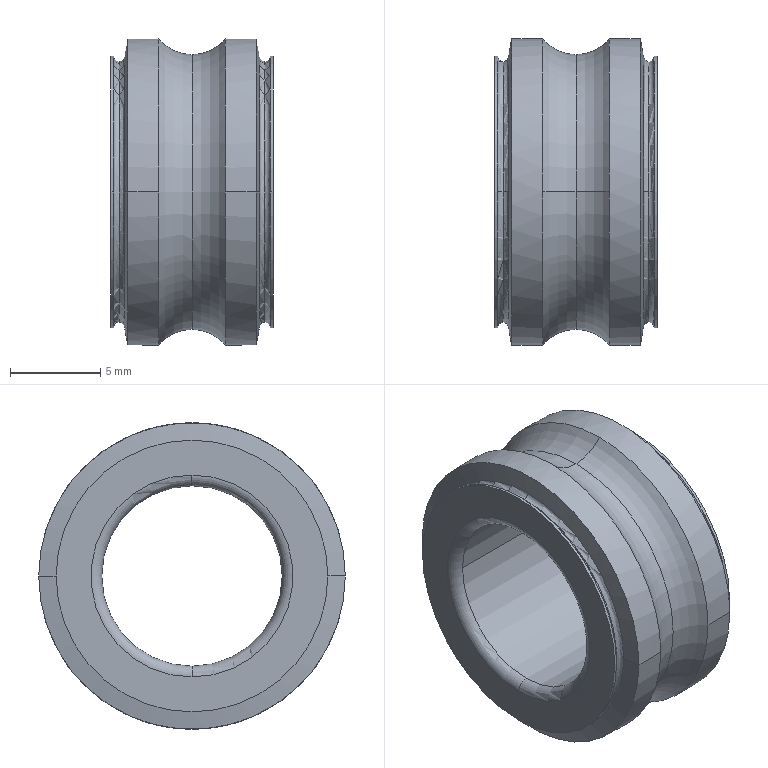Part | SolidWorks | features BaseBody 1 | 1 solid | 32 faces | box 9 x 17 x 17 mm | volume 1119 mm3 | torus 16 | cylinder 10 | cone 4 | plane 2 | commonest cylinder face diameters 15.07 x4 17 x4 10 x2
STEP:
#1=CARTESIAN_POINT('',(6.349,8.5,0.));
#2=VERTEX_POINT('',#1);
#3=CARTESIAN_POINT('',(8.065,8.5,0.));
#4=VERTEX_POINT('',#3);
#5=CARTESIAN_POINT('',(7.207,8.5,0.));
#6=DIRECTION('',(1.,0.,0.));
#7=VECTOR('',#6,1000.);
#8=LINE('',#5,#7);
#9=EDGE_CURVE('',#2,#4,#8,.T.);
#10=ORIENTED_EDGE('',*,*,#9,.T.);
#11=CARTESIAN_POINT('',(8.065,-8.5,0.));
#12=VERTEX_POINT('',#11);
#13=CARTESIAN_POINT('',(8.065,0.,0.));
#14=DIRECTION('',(1.,0.,0.));
#15=DIRECTION('',(0.,1.,0.));
#16=AXIS2_PLACEMENT_3D('',#13,#14,#15);
#17=CIRCLE('',#16,8.5);
#18=EDGE_CURVE('',#12,#4,#17,.T.);
#19=ORIENTED_EDGE('',*,*,#18,.F.);
#20=CARTESIAN_POINT('',(6.349,-8.5,0.));
#21=VERTEX_POINT('',#20);
#22=CARTESIAN_POINT('',(7.207,-8.5,0.));
#23=DIRECTION('',(-1.,0.,0.));
#24=VECTOR('',#23,1000.);
#25=LINE('',#22,#24);
#26=EDGE_CURVE('',#12,#21,#25,.T.);
#27=ORIENTED_EDGE('',*,*,#26,.T.);
#28=CARTESIAN_POINT('',(6.349,0.,-8.5));
#29=VERTEX_POINT('',#28);
#30=CARTESIAN_POINT('',(6.349,0.,0.));
#31=DIRECTION('',(1.,0.,0.));
#32=DIRECTION('',(0.,1.,0.));
#33=AXIS2_PLACEMENT_3D('',#30,#31,#32);
#34=CIRCLE('',#33,8.5);
#35=EDGE_CURVE('',#21,#29,#34,.T.);
#36=ORIENTED_EDGE('',*,*,#35,.T.);
#37=CARTESIAN_POINT('',(6.349,0.,0.));
#38=DIRECTION('',(1.,0.,0.));
#39=DIRECTION('',(0.,1.,0.));
#40=AXIS2_PLACEMENT_3D('',#37,#38,#39);
#41=CIRCLE('',#40,8.5);
#42=EDGE_CURVE('',#29,#2,#41,.T.);
#43=ORIENTED_EDGE('',*,*,#42,.T.);
#44=EDGE_LOOP('',(#10,#19,#27,#36,#43));
#45=FACE_OUTER_BOUND('',#44,.T.);
#46=CARTESIAN_POINT('',(7.207,0.,0.));
#47=DIRECTION('',(1.,0.,0.));
#48=DIRECTION('',(0.,1.,0.));
#49=AXIS2_PLACEMENT_3D('',#46,#47,#48);
#50=CYLINDRICAL_SURFACE('',#49,8.5);
#51=ADVANCED_FACE('',(#45),#50,.T.);
#52=CARTESIAN_POINT('',(4.5,0.,7.619));
#53=VERTEX_POINT('',#52);
#54=CARTESIAN_POINT('',(4.5,0.,-7.619));
#55=VERTEX_POINT('',#54);
#56=CARTESIAN_POINT('',(4.5,0.,0.));
#57=DIRECTION('',(-1.,0.,0.));
#58=DIRECTION('',(0.,0.,1.));
#59=AXIS2_PLACEMENT_3D('',#56,#57,#58);
#60=CIRCLE('',#59,7.619);
#61=EDGE_CURVE('',#53,#55,#60,.T.);
#62=ORIENTED_EDGE('',*,*,#61,.T.);
#63=CARTESIAN_POINT('',(2.651,0.,-8.5));
#64=VERTEX_POINT('',#63);
#65=CARTESIAN_POINT('',(4.5,0.,-10.));
#66=DIRECTION('',(0.,-1.,0.));
#67=DIRECTION('',(0.,0.,-1.));
#68=AXIS2_PLACEMENT_3D('',#65,#66,#67);
#69=CIRCLE('',#68,2.381);
#70=EDGE_CURVE('',#55,#64,#69,.T.);
#71=ORIENTED_EDGE('',*,*,#70,.T.);
#72=CARTESIAN_POINT('',(2.651,8.5,0.));
#73=VERTEX_POINT('',#72);
#74=CARTESIAN_POINT('',(2.651,0.,0.));
#75=DIRECTION('',(1.,0.,0.));
#76=DIRECTION('',(0.,1.,0.));
#77=AXIS2_PLACEMENT_3D('',#74,#75,#76);
#78=CIRCLE('',#77,8.5);
#79=EDGE_CURVE('',#64,#73,#78,.T.);
#80=ORIENTED_EDGE('',*,*,#79,.T.);
#81=CARTESIAN_POINT('',(2.651,0.,8.5));
#82=VERTEX_POINT('',#81);
#83=CARTESIAN_POINT('',(2.651,0.,0.));
#84=DIRECTION('',(1.,0.,0.));
#85=DIRECTION('',(0.,1.,0.));
#86=AXIS2_PLACEMENT_3D('',#83,#84,#85);
#87=CIRCLE('',#86,8.5);
#88=EDGE_CURVE('',#73,#82,#87,.T.);
#89=ORIENTED_EDGE('',*,*,#88,.T.);
#90=CARTESIAN_POINT('',(4.5,0.,10.));
#91=DIRECTION('',(0.,-1.,0.));
#92=DIRECTION('',(0.,0.,1.));
#93=AXIS2_PLACEMENT_3D('',#90,#91,#92);
#94=CIRCLE('',#93,2.381);
#95=EDGE_CURVE('',#82,#53,#94,.T.);
#96=ORIENTED_EDGE('',*,*,#95,.T.);
#97=EDGE_LOOP('',(#62,#71,#80,#89,#96));
#98=FACE_OUTER_BOUND('',#97,.T.);
#99=CARTESIAN_POINT('',(4.5,0.,0.));
#100=DIRECTION('',(1.,0.,0.));
#101=DIRECTION('',(0.,0.,-1.));
#102=AXIS2_PLACEMENT_3D('',#99,#100,#101);
#103=TOROIDAL_SURFACE('',#102,10.,2.381);
#104=ADVANCED_FACE('',(#98),#103,.F.);
#105=CARTESIAN_POINT('',(0.9348,8.5,0.));
#106=VERTEX_POINT('',#105);
#107=CARTESIAN_POINT('',(1.793,8.5,0.));
#108=DIRECTION('',(1.,0.,0.));
#109=VECTOR('',#108,1000.);
#110=LINE('',#107,#109);
#111=EDGE_CURVE('',#106,#73,#110,.T.);
#112=ORIENTED_EDGE('',*,*,#111,.T.);
#113=ORIENTED_EDGE('',*,*,#79,.F.);
#114=CARTESIAN_POINT('',(2.651,-8.5,0.));
#115=VERTEX_POINT('',#114);
#116=CARTESIAN_POINT('',(2.651,0.,0.));
#117=DIRECTION('',(1.,0.,0.));
#118=DIRECTION('',(0.,1.,0.));
#119=AXIS2_PLACEMENT_3D('',#116,#117,#118);
#120=CIRCLE('',#119,8.5);
#121=EDGE_CURVE('',#115,#64,#120,.T.);
#122=ORIENTED_EDGE('',*,*,#121,.F.);
#123=CARTESIAN_POINT('',(0.9348,-8.5,0.));
#124=VERTEX_POINT('',#123);
#125=CARTESIAN_POINT('',(1.793,-8.5,0.));
#126=DIRECTION('',(-1.,0.,0.));
#127=VECTOR('',#126,1000.);
#128=LINE('',#125,#127);
#129=EDGE_CURVE('',#115,#124,#128,.T.);
#130=ORIENTED_EDGE('',*,*,#129,.T.);
#131=CARTESIAN_POINT('',(0.9348,0.,0.));
#132=DIRECTION('',(1.,0.,0.));
#133=DIRECTION('',(0.,1.,0.));
#134=AXIS2_PLACEMENT_3D('',#131,#132,#133);
#135=CIRCLE('',#134,8.5);
#136=EDGE_CURVE('',#124,#106,#135,.T.);
#137=ORIENTED_EDGE('',*,*,#136,.T.);
#138=EDGE_LOOP('',(#112,#113,#122,#130,#137));
#139=FACE_OUTER_BOUND('',#138,.T.);
#140=CARTESIAN_POINT('',(1.793,0.,0.));
#141=DIRECTION('',(1.,0.,0.));
#142=DIRECTION('',(0.,1.,0.));
#143=AXIS2_PLACEMENT_3D('',#140,#141,#142);
#144=CYLINDRICAL_SURFACE('',#143,8.5);
#145=ADVANCED_FACE('',(#139),#144,.T.);
#146=CARTESIAN_POINT('',(0.7554,7.482,0.));
#147=VERTEX_POINT('',#146);
#148=CARTESIAN_POINT('',(0.8451,7.991,0.));
#149=DIRECTION('',(0.1736,0.9848,0.));
#150=VECTOR('',#149,1000.);
#151=LINE('',#148,#150);
#152=EDGE_CURVE('',#147,#106,#151,.T.);
#153=ORIENTED_EDGE('',*,*,#152,.T.);
#154=ORIENTED_EDGE('',*,*,#136,.F.);
#155=CARTESIAN_POINT('',(0.7554,-7.482,0.));
#156=VERTEX_POINT('',#155);
#157=CARTESIAN_POINT('',(0.8451,-7.991,0.));
#158=DIRECTION('',(-0.1736,0.9848,0.));
#159=VECTOR('',#158,1000.);
#160=LINE('',#157,#159);
#161=EDGE_CURVE('',#124,#156,#160,.T.);
#162=ORIENTED_EDGE('',*,*,#161,.T.);
#163=CARTESIAN_POINT('',(0.7554,0.,-7.482));
#164=VERTEX_POINT('',#163);
#165=CARTESIAN_POINT('',(0.7554,0.,0.));
#166=DIRECTION('',(1.,0.,0.));
#167=DIRECTION('',(0.,1.,0.));
#168=AXIS2_PLACEMENT_3D('',#165,#166,#167);
#169=CIRCLE('',#168,7.482);
#170=EDGE_CURVE('',#156,#164,#169,.T.);
#171=ORIENTED_EDGE('',*,*,#170,.T.);
#172=CARTESIAN_POINT('',(0.7554,0.,0.));
#173=DIRECTION('',(1.,0.,0.));
#174=DIRECTION('',(0.,1.,0.));
#175=AXIS2_PLACEMENT_3D('',#172,#173,#174);
#176=CIRCLE('',#175,7.482);
#177=EDGE_CURVE('',#164,#147,#176,.T.);
#178=ORIENTED_EDGE('',*,*,#177,.T.);
#179=EDGE_LOOP('',(#153,#154,#162,#171,#178));
#180=FACE_OUTER_BOUND('',#179,.T.);
#181=CARTESIAN_POINT('',(0.8451,0.,0.));
#182=DIRECTION('',(1.,0.,0.));
#183=DIRECTION('',(0.,1.,0.));
#184=AXIS2_PLACEMENT_3D('',#181,#182,#183);
#185=CONICAL_SURFACE('',#184,7.991,1.396);
#186=ADVANCED_FACE('',(#180),#185,.T.);
#187=CARTESIAN_POINT('',(0.456,0.,7.231));
#188=VERTEX_POINT('',#187);
#189=CARTESIAN_POINT('',(0.456,0.,-7.231));
#190=VERTEX_POINT('',#189);
#191=CARTESIAN_POINT('',(0.456,0.,0.));
#192=DIRECTION('',(-1.,0.,0.));
#193=DIRECTION('',(0.,0.,1.));
#194=AXIS2_PLACEMENT_3D('',#191,#192,#193);
#195=CIRCLE('',#194,7.231);
#196=EDGE_CURVE('',#188,#190,#195,.T.);
#197=ORIENTED_EDGE('',*,*,#196,.T.);
#198=CARTESIAN_POINT('',(0.152,0.,-7.535));
#199=VERTEX_POINT('',#198);
#200=CARTESIAN_POINT('',(0.456,0.,-7.535));
#201=DIRECTION('',(0.,-1.,0.));
#202=DIRECTION('',(0.,0.,-1.));
#203=AXIS2_PLACEMENT_3D('',#200,#201,#202);
#204=CIRCLE('',#203,0.304);
#205=EDGE_CURVE('',#190,#199,#204,.T.);
#206=ORIENTED_EDGE('',*,*,#205,.T.);
#207=CARTESIAN_POINT('',(0.152,7.535,0.));
#208=VERTEX_POINT('',#207);
#209=CARTESIAN_POINT('',(0.152,0.,0.));
#210=DIRECTION('',(1.,0.,0.));
#211=DIRECTION('',(0.,1.,0.));
#212=AXIS2_PLACEMENT_3D('',#209,#210,#211);
#213=CIRCLE('',#212,7.535);
#214=EDGE_CURVE('',#199,#208,#213,.T.);
#215=ORIENTED_EDGE('',*,*,#214,.T.);
#216=CARTESIAN_POINT('',(0.152,0.,7.535));
#217=VERTEX_POINT('',#216);
#218=CARTESIAN_POINT('',(0.152,0.,0.));
#219=DIRECTION('',(1.,0.,0.));
#220=DIRECTION('',(0.,1.,0.));
#221=AXIS2_PLACEMENT_3D('',#218,#219,#220);
#222=CIRCLE('',#221,7.535);
#223=EDGE_CURVE('',#208,#217,#222,.T.);
#224=ORIENTED_EDGE('',*,*,#223,.T.);
#225=CARTESIAN_POINT('',(0.456,0.,7.535));
#226=DIRECTION('',(0.,-1.,0.));
#227=DIRECTION('',(0.,0.,1.));
#228=AXIS2_PLACEMENT_3D('',#225,#226,#227);
#229=CIRCLE('',#228,0.304);
#230=EDGE_CURVE('',#217,#188,#229,.T.);
#231=ORIENTED_EDGE('',*,*,#230,.T.);
#232=EDGE_LOOP('',(#197,#206,#215,#224,#231));
#233=FACE_OUTER_BOUND('',#232,.T.);
#234=CARTESIAN_POINT('',(0.456,0.,0.));
#235=DIRECTION('',(1.,0.,0.));
#236=DIRECTION('',(0.,0.,-1.));
#237=AXIS2_PLACEMENT_3D('',#234,#235,#236);
#238=TOROIDAL_SURFACE('',#237,7.535,0.304);
#239=ADVANCED_FACE('',(#233),#238,.F.);
#240=CARTESIAN_POINT('',(0.,7.535,0.));
#241=VERTEX_POINT('',#240);
#242=CARTESIAN_POINT('',(0.076,7.535,0.));
#243=DIRECTION('',(1.,0.,0.));
#244=VECTOR('',#243,1000.);
#245=LINE('',#242,#244);
#246=EDGE_CURVE('',#241,#208,#245,.T.);
#247=ORIENTED_EDGE('',*,*,#246,.T.);
#248=ORIENTED_EDGE('',*,*,#214,.F.);
#249=CARTESIAN_POINT('',(0.152,-7.535,0.));
#250=VERTEX_POINT('',#249);
#251=CARTESIAN_POINT('',(0.152,0.,0.));
#252=DIRECTION('',(1.,0.,0.));
#253=DIRECTION('',(0.,1.,0.));
#254=AXIS2_PLACEMENT_3D('',#251,#252,#253);
#255=CIRCLE('',#254,7.535);
#256=EDGE_CURVE('',#250,#199,#255,.T.);
#257=ORIENTED_EDGE('',*,*,#256,.F.);
#258=CARTESIAN_POINT('',(0.,-7.535,0.));
#259=VERTEX_POINT('',#258);
#260=CARTESIAN_POINT('',(0.076,-7.535,0.));
#261=DIRECTION('',(-1.,0.,0.));
#262=VECTOR('',#261,1000.);
#263=LINE('',#260,#262);
#264=EDGE_CURVE('',#250,#259,#263,.T.);
#265=ORIENTED_EDGE('',*,*,#264,.T.);
#266=CARTESIAN_POINT('',(0.,0.,0.));
#267=DIRECTION('',(1.,0.,0.));
#268=DIRECTION('',(0.,1.,0.));
#269=AXIS2_PLACEMENT_3D('',#266,#267,#268);
#270=CIRCLE('',#269,7.535);
#271=EDGE_CURVE('',#259,#241,#270,.T.);
#272=ORIENTED_EDGE('',*,*,#271,.T.);
#273=EDGE_LOOP('',(#247,#248,#257,#265,#272));
#274=FACE_OUTER_BOUND('',#273,.T.);
#275=CARTESIAN_POINT('',(0.076,0.,0.));
#276=DIRECTION('',(1.,0.,0.));
#277=DIRECTION('',(0.,1.,0.));
#278=AXIS2_PLACEMENT_3D('',#275,#276,#277);
#279=CYLINDRICAL_SURFACE('',#278,7.535);
#280=ADVANCED_FACE('',(#274),#279,.T.);
#281=CARTESIAN_POINT('',(0.,0.,5.6));
#282=VERTEX_POINT('',#281);
#283=CARTESIAN_POINT('',(0.,0.,-5.6));
#284=VERTEX_POINT('',#283);
#285=CARTESIAN_POINT('',(0.,0.,0.));
#286=DIRECTION('',(1.,0.,0.));
#287=DIRECTION('',(0.,1.,0.));
#288=AXIS2_PLACEMENT_3D('',#285,#286,#287);
#289=CIRCLE('',#288,5.6);
#290=EDGE_CURVE('',#282,#284,#289,.T.);
#291=ORIENTED_EDGE('',*,*,#290,.T.);
#292=CARTESIAN_POINT('',(0.,0.,0.));
#293=DIRECTION('',(1.,0.,0.));
#294=DIRECTION('',(0.,1.,0.));
#295=AXIS2_PLACEMENT_3D('',#292,#293,#294);
#296=CIRCLE('',#295,5.6);
#297=EDGE_CURVE('',#284,#282,#296,.T.);
#298=ORIENTED_EDGE('',*,*,#297,.T.);
#299=EDGE_LOOP('',(#291,#298));
#300=FACE_BOUND('',#299,.T.);
#301=CARTESIAN_POINT('',(0.,0.,0.));
#302=DIRECTION('',(1.,0.,0.));
#303=DIRECTION('',(0.,1.,0.));
#304=AXIS2_PLACEMENT_3D('',#301,#302,#303);
#305=CIRCLE('',#304,7.535);
#306=EDGE_CURVE('',#241,#259,#305,.T.);
#307=ORIENTED_EDGE('',*,*,#306,.F.);
#308=ORIENTED_EDGE('',*,*,#271,.F.);
#309=EDGE_LOOP('',(#307,#308));
#310=FACE_OUTER_BOUND('',#309,.T.);
#311=CARTESIAN_POINT('',(0.,6.568,0.));
#312=DIRECTION('',(-1.,0.,0.));
#313=DIRECTION('',(0.,0.,1.));
#314=AXIS2_PLACEMENT_3D('',#311,#312,#313);
#315=PLANE('',#314);
#316=ADVANCED_FACE('',(#300,#310),#315,.T.);
#317=CARTESIAN_POINT('',(0.6,0.,-5.));
#318=VERTEX_POINT('',#317);
#319=CARTESIAN_POINT('',(0.6,0.,-5.6));
#320=DIRECTION('',(0.,-1.,0.));
#321=DIRECTION('',(0.,0.,-1.));
#322=AXIS2_PLACEMENT_3D('',#319,#320,#321);
#323=CIRCLE('',#322,0.6);
#324=EDGE_CURVE('',#318,#284,#323,.T.);
#325=ORIENTED_EDGE('',*,*,#324,.T.);
#326=ORIENTED_EDGE('',*,*,#290,.F.);
#327=CARTESIAN_POINT('',(0.6,0.,5.));
#328=VERTEX_POINT('',#327);
#329=CARTESIAN_POINT('',(0.6,0.,5.6));
#330=DIRECTION('',(0.,-1.,0.));
#331=DIRECTION('',(0.,0.,1.));
#332=AXIS2_PLACEMENT_3D('',#329,#330,#331);
#333=CIRCLE('',#332,0.6);
#334=EDGE_CURVE('',#282,#328,#333,.T.);
#335=ORIENTED_EDGE('',*,*,#334,.T.);
#336=CARTESIAN_POINT('',(0.6,-5.,0.));
#337=VERTEX_POINT('',#336);
#338=CARTESIAN_POINT('',(0.6,0.,0.));
#339=DIRECTION('',(1.,0.,0.));
#340=DIRECTION('',(0.,1.,0.));
#341=AXIS2_PLACEMENT_3D('',#338,#339,#340);
#342=CIRCLE('',#341,5.);
#343=EDGE_CURVE('',#328,#337,#342,.T.);
#344=ORIENTED_EDGE('',*,*,#343,.T.);
#345=CARTESIAN_POINT('',(0.6,0.,0.));
#346=DIRECTION('',(1.,0.,0.));
#347=DIRECTION('',(0.,1.,0.));
#348=AXIS2_PLACEMENT_3D('',#345,#346,#347);
#349=CIRCLE('',#348,5.);
#350=EDGE_CURVE('',#337,#318,#349,.T.);
#351=ORIENTED_EDGE('',*,*,#350,.T.);
#352=EDGE_LOOP('',(#325,#326,#335,#344,#351));
#353=FACE_OUTER_BOUND('',#352,.T.);
#354=CARTESIAN_POINT('',(0.6,0.,0.));
#355=DIRECTION('',(1.,0.,0.));
#356=DIRECTION('',(0.,0.,-1.));
#357=AXIS2_PLACEMENT_3D('',#354,#355,#356);
#358=TOROIDAL_SURFACE('',#357,5.6,0.6);
#359=ADVANCED_FACE('',(#353),#358,.T.);
#360=CARTESIAN_POINT('',(0.6,5.,0.));
#361=VERTEX_POINT('',#360);
#362=CARTESIAN_POINT('',(8.4,5.,0.));
#363=VERTEX_POINT('',#362);
#364=CARTESIAN_POINT('',(4.5,5.,0.));
#365=DIRECTION('',(1.,0.,0.));
#366=VECTOR('',#365,1000.);
#367=LINE('',#364,#366);
#368=EDGE_CURVE('',#361,#363,#367,.T.);
#369=ORIENTED_EDGE('',*,*,#368,.T.);
#370=CARTESIAN_POINT('',(8.4,0.,5.));
#371=VERTEX_POINT('',#370);
#372=CARTESIAN_POINT('',(8.4,0.,0.));
#373=DIRECTION('',(1.,0.,0.));
#374=DIRECTION('',(0.,1.,0.));
#375=AXIS2_PLACEMENT_3D('',#372,#373,#374);
#376=CIRCLE('',#375,5.);
#377=EDGE_CURVE('',#363,#371,#376,.T.);
#378=ORIENTED_EDGE('',*,*,#377,.T.);
#379=CARTESIAN_POINT('',(8.4,-5.,0.));
#380=VERTEX_POINT('',#379);
#381=CARTESIAN_POINT('',(8.4,0.,0.));
#382=DIRECTION('',(1.,0.,0.));
#383=DIRECTION('',(0.,1.,0.));
#384=AXIS2_PLACEMENT_3D('',#381,#382,#383);
#385=CIRCLE('',#384,5.);
#386=EDGE_CURVE('',#371,#380,#385,.T.);
#387=ORIENTED_EDGE('',*,*,#386,.T.);
#388=CARTESIAN_POINT('',(4.5,-5.,0.));
#389=DIRECTION('',(-1.,0.,0.));
#390=VECTOR('',#389,1000.);
#391=LINE('',#388,#390);
#392=EDGE_CURVE('',#380,#337,#391,.T.);
#393=ORIENTED_EDGE('',*,*,#392,.T.);
#394=ORIENTED_EDGE('',*,*,#343,.F.);
#395=CARTESIAN_POINT('',(0.6,0.,0.));
#396=DIRECTION('',(1.,0.,0.));
#397=DIRECTION('',(0.,1.,0.));
#398=AXIS2_PLACEMENT_3D('',#395,#396,#397);
#399=CIRCLE('',#398,5.);
#400=EDGE_CURVE('',#361,#328,#399,.T.);
#401=ORIENTED_EDGE('',*,*,#400,.F.);
#402=EDGE_LOOP('',(#369,#378,#387,#393,#394,#401));
#403=FACE_OUTER_BOUND('',#402,.T.);
#404=CARTESIAN_POINT('',(4.5,0.,0.));
#405=DIRECTION('',(1.,0.,0.));
#406=DIRECTION('',(0.,1.,0.));
#407=AXIS2_PLACEMENT_3D('',#404,#405,#406);
#408=CYLINDRICAL_SURFACE('',#407,5.);
#409=ADVANCED_FACE('',(#403),#408,.F.);
#410=CARTESIAN_POINT('',(9.,0.,-5.6));
#411=VERTEX_POINT('',#410);
#412=CARTESIAN_POINT('',(8.4,0.,-5.));
#413=VERTEX_POINT('',#412);
#414=CARTESIAN_POINT('',(8.4,0.,-5.6));
#415=DIRECTION('',(0.,-1.,0.));
#416=DIRECTION('',(0.,0.,-1.));
#417=AXIS2_PLACEMENT_3D('',#414,#415,#416);
#418=CIRCLE('',#417,0.6);
#419=EDGE_CURVE('',#411,#413,#418,.T.);
#420=ORIENTED_EDGE('',*,*,#419,.T.);
#421=CARTESIAN_POINT('',(8.4,0.,0.));
#422=DIRECTION('',(1.,0.,0.));
#423=DIRECTION('',(0.,1.,0.));
#424=AXIS2_PLACEMENT_3D('',#421,#422,#423);
#425=CIRCLE('',#424,5.);
#426=EDGE_CURVE('',#380,#413,#425,.T.);
#427=ORIENTED_EDGE('',*,*,#426,.F.);
#428=ORIENTED_EDGE('',*,*,#386,.F.);
#429=CARTESIAN_POINT('',(9.,0.,5.6));
#430=VERTEX_POINT('',#429);
#431=CARTESIAN_POINT('',(8.4,0.,5.6));
#432=DIRECTION('',(0.,-1.,0.));
#433=DIRECTION('',(0.,0.,1.));
#434=AXIS2_PLACEMENT_3D('',#431,#432,#433);
#435=CIRCLE('',#434,0.6);
#436=EDGE_CURVE('',#371,#430,#435,.T.);
#437=ORIENTED_EDGE('',*,*,#436,.T.);
#438=CARTESIAN_POINT('',(9.,0.,0.));
#439=DIRECTION('',(1.,0.,0.));
#440=DIRECTION('',(0.,1.,0.));
#441=AXIS2_PLACEMENT_3D('',#438,#439,#440);
#442=CIRCLE('',#441,5.6);
#443=EDGE_CURVE('',#430,#411,#442,.T.);
#444=ORIENTED_EDGE('',*,*,#443,.T.);
#445=EDGE_LOOP('',(#420,#427,#428,#437,#444));
#446=FACE_OUTER_BOUND('',#445,.T.);
#447=CARTESIAN_POINT('',(8.4,0.,0.));
#448=DIRECTION('',(1.,0.,0.));
#449=DIRECTION('',(0.,0.,-1.));
#450=AXIS2_PLACEMENT_3D('',#447,#448,#449);
#451=TOROIDAL_SURFACE('',#450,5.6,0.6);
#452=ADVANCED_FACE('',(#446),#451,.T.);
#453=CARTESIAN_POINT('',(9.,0.,0.));
#454=DIRECTION('',(1.,0.,0.));
#455=DIRECTION('',(0.,1.,0.));
#456=AXIS2_PLACEMENT_3D('',#453,#454,#455);
#457=CIRCLE('',#456,5.6);
#458=EDGE_CURVE('',#411,#430,#457,.T.);
#459=ORIENTED_EDGE('',*,*,#458,.F.);
#460=ORIENTED_EDGE('',*,*,#443,.F.);
#461=EDGE_LOOP('',(#459,#460));
#462=FACE_BOUND('',#461,.T.);
#463=CARTESIAN_POINT('',(9.,7.535,0.));
#464=VERTEX_POINT('',#463);
#465=CARTESIAN_POINT('',(9.,-7.535,0.));
#466=VERTEX_POINT('',#465);
#467=CARTESIAN_POINT('',(9.,0.,0.));
#468=DIRECTION('',(1.,0.,0.));
#469=DIRECTION('',(0.,1.,0.));
#470=AXIS2_PLACEMENT_3D('',#467,#468,#469);
#471=CIRCLE('',#470,7.535);
#472=EDGE_CURVE('',#464,#466,#471,.T.);
#473=ORIENTED_EDGE('',*,*,#472,.T.);
#474=CARTESIAN_POINT('',(9.,0.,0.));
#475=DIRECTION('',(1.,0.,0.));
#476=DIRECTION('',(0.,1.,0.));
#477=AXIS2_PLACEMENT_3D('',#474,#475,#476);
#478=CIRCLE('',#477,7.535);
#479=EDGE_CURVE('',#466,#464,#478,.T.);
#480=ORIENTED_EDGE('',*,*,#479,.T.);
#481=EDGE_LOOP('',(#473,#480));
#482=FACE_OUTER_BOUND('',#481,.T.);
#483=CARTESIAN_POINT('',(9.,6.568,0.));
#484=DIRECTION('',(1.,0.,0.));
#485=DIRECTION('',(0.,1.,0.));
#486=AXIS2_PLACEMENT_3D('',#483,#484,#485);
#487=PLANE('',#486);
#488=ADVANCED_FACE('',(#462,#482),#487,.T.);
#489=CARTESIAN_POINT('',(8.848,7.535,0.));
#490=VERTEX_POINT('',#489);
#491=CARTESIAN_POINT('',(8.924,7.535,0.));
#492=DIRECTION('',(1.,0.,0.));
#493=VECTOR('',#492,1000.);
#494=LINE('',#491,#493);
#495=EDGE_CURVE('',#490,#464,#494,.T.);
#496=ORIENTED_EDGE('',*,*,#495,.T.);
#497=ORIENTED_EDGE('',*,*,#479,.F.);
#498=CARTESIAN_POINT('',(8.848,-7.535,0.));
#499=VERTEX_POINT('',#498);
#500=CARTESIAN_POINT('',(8.924,-7.535,0.));
#501=DIRECTION('',(-1.,0.,0.));
#502=VECTOR('',#501,1000.);
#503=LINE('',#500,#502);
#504=EDGE_CURVE('',#466,#499,#503,.T.);
#505=ORIENTED_EDGE('',*,*,#504,.T.);
#506=CARTESIAN_POINT('',(8.848,0.,-7.535));
#507=VERTEX_POINT('',#506);
#508=CARTESIAN_POINT('',(8.848,0.,0.));
#509=DIRECTION('',(1.,0.,0.));
#510=DIRECTION('',(0.,1.,0.));
#511=AXIS2_PLACEMENT_3D('',#508,#509,#510);
#512=CIRCLE('',#511,7.535);
#513=EDGE_CURVE('',#499,#507,#512,.T.);
#514=ORIENTED_EDGE('',*,*,#513,.T.);
#515=CARTESIAN_POINT('',(8.848,0.,0.));
#516=DIRECTION('',(1.,0.,0.));
#517=DIRECTION('',(0.,1.,0.));
#518=AXIS2_PLACEMENT_3D('',#515,#516,#517);
#519=CIRCLE('',#518,7.535);
#520=EDGE_CURVE('',#507,#490,#519,.T.);
#521=ORIENTED_EDGE('',*,*,#520,.T.);
#522=EDGE_LOOP('',(#496,#497,#505,#514,#521));
#523=FACE_OUTER_BOUND('',#522,.T.);
#524=CARTESIAN_POINT('',(8.924,0.,0.));
#525=DIRECTION('',(1.,0.,0.));
#526=DIRECTION('',(0.,1.,0.));
#527=AXIS2_PLACEMENT_3D('',#524,#525,#526);
#528=CYLINDRICAL_SURFACE('',#527,7.535);
#529=ADVANCED_FACE('',(#523),#528,.T.);
#530=CARTESIAN_POINT('',(8.544,0.,7.231));
#531=VERTEX_POINT('',#530);
#532=CARTESIAN_POINT('',(8.544,0.,-7.231));
#533=VERTEX_POINT('',#532);
#534=CARTESIAN_POINT('',(8.544,0.,0.));
#535=DIRECTION('',(-1.,0.,0.));
#536=DIRECTION('',(0.,0.,1.));
#537=AXIS2_PLACEMENT_3D('',#534,#535,#536);
#538=CIRCLE('',#537,7.231);
#539=EDGE_CURVE('',#531,#533,#538,.T.);
#540=ORIENTED_EDGE('',*,*,#539,.T.);
#541=CARTESIAN_POINT('',(8.245,0.,-7.482));
#542=VERTEX_POINT('',#541);
#543=CARTESIAN_POINT('',(8.544,0.,-7.535));
#544=DIRECTION('',(0.,-1.,0.));
#545=DIRECTION('',(0.,0.,-1.));
#546=AXIS2_PLACEMENT_3D('',#543,#544,#545);
#547=CIRCLE('',#546,0.304);
#548=EDGE_CURVE('',#533,#542,#547,.T.);
#549=ORIENTED_EDGE('',*,*,#548,.T.);
#550=CARTESIAN_POINT('',(8.245,7.482,0.));
#551=VERTEX_POINT('',#550);
#552=CARTESIAN_POINT('',(8.245,0.,0.));
#553=DIRECTION('',(1.,0.,0.));
#554=DIRECTION('',(0.,1.,0.));
#555=AXIS2_PLACEMENT_3D('',#552,#553,#554);
#556=CIRCLE('',#555,7.482);
#557=EDGE_CURVE('',#542,#551,#556,.T.);
#558=ORIENTED_EDGE('',*,*,#557,.T.);
#559=CARTESIAN_POINT('',(8.245,0.,7.482));
#560=VERTEX_POINT('',#559);
#561=CARTESIAN_POINT('',(8.245,0.,0.));
#562=DIRECTION('',(1.,0.,0.));
#563=DIRECTION('',(0.,1.,0.));
#564=AXIS2_PLACEMENT_3D('',#561,#562,#563);
#565=CIRCLE('',#564,7.482);
#566=EDGE_CURVE('',#551,#560,#565,.T.);
#567=ORIENTED_EDGE('',*,*,#566,.T.);
#568=CARTESIAN_POINT('',(8.544,0.,7.535));
#569=DIRECTION('',(0.,-1.,0.));
#570=DIRECTION('',(0.,0.,1.));
#571=AXIS2_PLACEMENT_3D('',#568,#569,#570);
#572=CIRCLE('',#571,0.304);
#573=EDGE_CURVE('',#560,#531,#572,.T.);
#574=ORIENTED_EDGE('',*,*,#573,.T.);
#575=EDGE_LOOP('',(#540,#549,#558,#567,#574));
#576=FACE_OUTER_BOUND('',#575,.T.);
#577=CARTESIAN_POINT('',(8.544,0.,0.));
#578=DIRECTION('',(1.,0.,0.));
#579=DIRECTION('',(0.,0.,-1.));
#580=AXIS2_PLACEMENT_3D('',#577,#578,#579);
#581=TOROIDAL_SURFACE('',#580,7.535,0.304);
#582=ADVANCED_FACE('',(#576),#581,.F.);
#583=CARTESIAN_POINT('',(8.155,7.991,0.));
#584=DIRECTION('',(0.1736,-0.9848,0.));
#585=VECTOR('',#584,1000.);
#586=LINE('',#583,#585);
#587=EDGE_CURVE('',#4,#551,#586,.T.);
#588=ORIENTED_EDGE('',*,*,#587,.T.);
#589=ORIENTED_EDGE('',*,*,#557,.F.);
#590=CARTESIAN_POINT('',(8.245,-7.482,0.));
#591=VERTEX_POINT('',#590);
#592=CARTESIAN_POINT('',(8.245,0.,0.));
#593=DIRECTION('',(1.,0.,0.));
#594=DIRECTION('',(0.,1.,0.));
#595=AXIS2_PLACEMENT_3D('',#592,#593,#594);
#596=CIRCLE('',#595,7.482);
#597=EDGE_CURVE('',#591,#542,#596,.T.);
#598=ORIENTED_EDGE('',*,*,#597,.F.);
#599=CARTESIAN_POINT('',(8.155,-7.991,0.));
#600=DIRECTION('',(-0.1736,-0.9848,0.));
#601=VECTOR('',#600,1000.);
#602=LINE('',#599,#601);
#603=EDGE_CURVE('',#591,#12,#602,.T.);
#604=ORIENTED_EDGE('',*,*,#603,.T.);
#605=ORIENTED_EDGE('',*,*,#18,.T.);
#606=EDGE_LOOP('',(#588,#589,#598,#604,#605));
#607=FACE_OUTER_BOUND('',#606,.T.);
#608=CARTESIAN_POINT('',(8.155,0.,0.));
#609=DIRECTION('',(-1.,0.,0.));
#610=DIRECTION('',(0.,1.,0.));
#611=AXIS2_PLACEMENT_3D('',#608,#609,#610);
#612=CONICAL_SURFACE('',#611,7.991,1.396);
#613=ADVANCED_FACE('',(#607),#612,.T.);
#614=ORIENTED_EDGE('',*,*,#587,.F.);
#615=CARTESIAN_POINT('',(8.065,0.,0.));
#616=DIRECTION('',(1.,0.,0.));
#617=DIRECTION('',(0.,1.,0.));
#618=AXIS2_PLACEMENT_3D('',#615,#616,#617);
#619=CIRCLE('',#618,8.5);
#620=EDGE_CURVE('',#4,#12,#619,.T.);
#621=ORIENTED_EDGE('',*,*,#620,.T.);
#622=ORIENTED_EDGE('',*,*,#603,.F.);
#623=CARTESIAN_POINT('',(8.245,0.,0.));
#624=DIRECTION('',(1.,0.,0.));
#625=DIRECTION('',(0.,1.,0.));
#626=AXIS2_PLACEMENT_3D('',#623,#624,#625);
#627=CIRCLE('',#626,7.482);
#628=EDGE_CURVE('',#560,#591,#627,.T.);
#629=ORIENTED_EDGE('',*,*,#628,.F.);
#630=ORIENTED_EDGE('',*,*,#566,.F.);
#631=EDGE_LOOP('',(#614,#621,#622,#629,#630));
#632=FACE_OUTER_BOUND('',#631,.T.);
#633=CARTESIAN_POINT('',(8.155,0.,0.));
#634=DIRECTION('',(-1.,0.,0.));
#635=DIRECTION('',(0.,1.,0.));
#636=AXIS2_PLACEMENT_3D('',#633,#634,#635);
#637=CONICAL_SURFACE('',#636,7.991,1.396);
#638=ADVANCED_FACE('',(#632),#637,.T.);
#639=CARTESIAN_POINT('',(8.544,0.,0.));
#640=DIRECTION('',(-1.,0.,0.));
#641=DIRECTION('',(0.,0.,1.));
#642=AXIS2_PLACEMENT_3D('',#639,#640,#641);
#643=CIRCLE('',#642,7.231);
#644=EDGE_CURVE('',#533,#531,#643,.T.);
#645=ORIENTED_EDGE('',*,*,#644,.T.);
#646=ORIENTED_EDGE('',*,*,#573,.F.);
#647=ORIENTED_EDGE('',*,*,#628,.T.);
#648=ORIENTED_EDGE('',*,*,#597,.T.);
#649=ORIENTED_EDGE('',*,*,#548,.F.);
#650=EDGE_LOOP('',(#645,#646,#647,#648,#649));
#651=FACE_OUTER_BOUND('',#650,.T.);
#652=CARTESIAN_POINT('',(8.544,0.,0.));
#653=DIRECTION('',(1.,0.,0.));
#654=DIRECTION('',(0.,0.,-1.));
#655=AXIS2_PLACEMENT_3D('',#652,#653,#654);
#656=TOROIDAL_SURFACE('',#655,7.535,0.304);
#657=ADVANCED_FACE('',(#651),#656,.F.);
#658=ORIENTED_EDGE('',*,*,#495,.F.);
#659=CARTESIAN_POINT('',(8.848,0.,7.535));
#660=VERTEX_POINT('',#659);
#661=CARTESIAN_POINT('',(8.848,0.,0.));
#662=DIRECTION('',(1.,0.,0.));
#663=DIRECTION('',(0.,1.,0.));
#664=AXIS2_PLACEMENT_3D('',#661,#662,#663);
#665=CIRCLE('',#664,7.535);
#666=EDGE_CURVE('',#490,#660,#665,.T.);
#667=ORIENTED_EDGE('',*,*,#666,.T.);
#668=CARTESIAN_POINT('',(8.848,0.,0.));
#669=DIRECTION('',(1.,0.,0.));
#670=DIRECTION('',(0.,1.,0.));
#671=AXIS2_PLACEMENT_3D('',#668,#669,#670);
#672=CIRCLE('',#671,7.535);
#673=EDGE_CURVE('',#660,#499,#672,.T.);
#674=ORIENTED_EDGE('',*,*,#673,.T.);
#675=ORIENTED_EDGE('',*,*,#504,.F.);
#676=ORIENTED_EDGE('',*,*,#472,.F.);
#677=EDGE_LOOP('',(#658,#667,#674,#675,#676));
#678=FACE_OUTER_BOUND('',#677,.T.);
#679=CARTESIAN_POINT('',(8.924,0.,0.));
#680=DIRECTION('',(1.,0.,0.));
#681=DIRECTION('',(0.,1.,0.));
#682=AXIS2_PLACEMENT_3D('',#679,#680,#681);
#683=CYLINDRICAL_SURFACE('',#682,7.535);
#684=ADVANCED_FACE('',(#678),#683,.T.);
#685=ORIENTED_EDGE('',*,*,#419,.F.);
#686=ORIENTED_EDGE('',*,*,#458,.T.);
#687=ORIENTED_EDGE('',*,*,#436,.F.);
#688=ORIENTED_EDGE('',*,*,#377,.F.);
#689=CARTESIAN_POINT('',(8.4,0.,0.));
#690=DIRECTION('',(1.,0.,0.));
#691=DIRECTION('',(0.,1.,0.));
#692=AXIS2_PLACEMENT_3D('',#689,#690,#691);
#693=CIRCLE('',#692,5.);
#694=EDGE_CURVE('',#413,#363,#693,.T.);
#695=ORIENTED_EDGE('',*,*,#694,.F.);
#696=EDGE_LOOP('',(#685,#686,#687,#688,#695));
#697=FACE_OUTER_BOUND('',#696,.T.);
#698=CARTESIAN_POINT('',(8.4,0.,0.));
#699=DIRECTION('',(1.,0.,0.));
#700=DIRECTION('',(0.,0.,-1.));
#701=AXIS2_PLACEMENT_3D('',#698,#699,#700);
#702=TOROIDAL_SURFACE('',#701,5.6,0.6);
#703=ADVANCED_FACE('',(#697),#702,.T.);
#704=ORIENTED_EDGE('',*,*,#368,.F.);
#705=CARTESIAN_POINT('',(0.6,0.,0.));
#706=DIRECTION('',(1.,0.,0.));
#707=DIRECTION('',(0.,1.,0.));
#708=AXIS2_PLACEMENT_3D('',#705,#706,#707);
#709=CIRCLE('',#708,5.);
#710=EDGE_CURVE('',#318,#361,#709,.T.);
#711=ORIENTED_EDGE('',*,*,#710,.F.);
#712=ORIENTED_EDGE('',*,*,#350,.F.);
#713=ORIENTED_EDGE('',*,*,#392,.F.);
#714=ORIENTED_EDGE('',*,*,#426,.T.);
#715=ORIENTED_EDGE('',*,*,#694,.T.);
#716=EDGE_LOOP('',(#704,#711,#712,#713,#714,#715));
#717=FACE_OUTER_BOUND('',#716,.T.);
#718=CARTESIAN_POINT('',(4.5,0.,0.));
#719=DIRECTION('',(1.,0.,0.));
#720=DIRECTION('',(0.,1.,0.));
#721=AXIS2_PLACEMENT_3D('',#718,#719,#720);
#722=CYLINDRICAL_SURFACE('',#721,5.);
#723=ADVANCED_FACE('',(#717),#722,.F.);
#724=ORIENTED_EDGE('',*,*,#324,.F.);
#725=ORIENTED_EDGE('',*,*,#710,.T.);
#726=ORIENTED_EDGE('',*,*,#400,.T.);
#727=ORIENTED_EDGE('',*,*,#334,.F.);
#728=ORIENTED_EDGE('',*,*,#297,.F.);
#729=EDGE_LOOP('',(#724,#725,#726,#727,#728));
#730=FACE_OUTER_BOUND('',#729,.T.);
#731=CARTESIAN_POINT('',(0.6,0.,0.));
#732=DIRECTION('',(1.,0.,0.));
#733=DIRECTION('',(0.,0.,-1.));
#734=AXIS2_PLACEMENT_3D('',#731,#732,#733);
#735=TOROIDAL_SURFACE('',#734,5.6,0.6);
#736=ADVANCED_FACE('',(#730),#735,.T.);
#737=ORIENTED_EDGE('',*,*,#246,.F.);
#738=ORIENTED_EDGE('',*,*,#306,.T.);
#739=ORIENTED_EDGE('',*,*,#264,.F.);
#740=CARTESIAN_POINT('',(0.152,0.,0.));
#741=DIRECTION('',(1.,0.,0.));
#742=DIRECTION('',(0.,1.,0.));
#743=AXIS2_PLACEMENT_3D('',#740,#741,#742);
#744=CIRCLE('',#743,7.535);
#745=EDGE_CURVE('',#217,#250,#744,.T.);
#746=ORIENTED_EDGE('',*,*,#745,.F.);
#747=ORIENTED_EDGE('',*,*,#223,.F.);
#748=EDGE_LOOP('',(#737,#738,#739,#746,#747));
#749=FACE_OUTER_BOUND('',#748,.T.);
#750=CARTESIAN_POINT('',(0.076,0.,0.));
#751=DIRECTION('',(1.,0.,0.));
#752=DIRECTION('',(0.,1.,0.));
#753=AXIS2_PLACEMENT_3D('',#750,#751,#752);
#754=CYLINDRICAL_SURFACE('',#753,7.535);
#755=ADVANCED_FACE('',(#749),#754,.T.);
#756=CARTESIAN_POINT('',(0.456,0.,0.));
#757=DIRECTION('',(-1.,0.,0.));
#758=DIRECTION('',(0.,0.,1.));
#759=AXIS2_PLACEMENT_3D('',#756,#757,#758);
#760=CIRCLE('',#759,7.231);
#761=EDGE_CURVE('',#190,#188,#760,.T.);
#762=ORIENTED_EDGE('',*,*,#761,.T.);
#763=ORIENTED_EDGE('',*,*,#230,.F.);
#764=ORIENTED_EDGE('',*,*,#745,.T.);
#765=ORIENTED_EDGE('',*,*,#256,.T.);
#766=ORIENTED_EDGE('',*,*,#205,.F.);
#767=EDGE_LOOP('',(#762,#763,#764,#765,#766));
#768=FACE_OUTER_BOUND('',#767,.T.);
#769=CARTESIAN_POINT('',(0.456,0.,0.));
#770=DIRECTION('',(1.,0.,0.));
#771=DIRECTION('',(0.,0.,-1.));
#772=AXIS2_PLACEMENT_3D('',#769,#770,#771);
#773=TOROIDAL_SURFACE('',#772,7.535,0.304);
#774=ADVANCED_FACE('',(#768),#773,.F.);
#775=ORIENTED_EDGE('',*,*,#152,.F.);
#776=CARTESIAN_POINT('',(0.7554,0.,7.482));
#777=VERTEX_POINT('',#776);
#778=CARTESIAN_POINT('',(0.7554,0.,0.));
#779=DIRECTION('',(1.,0.,0.));
#780=DIRECTION('',(0.,1.,0.));
#781=AXIS2_PLACEMENT_3D('',#778,#779,#780);
#782=CIRCLE('',#781,7.482);
#783=EDGE_CURVE('',#147,#777,#782,.T.);
#784=ORIENTED_EDGE('',*,*,#783,.T.);
#785=CARTESIAN_POINT('',(0.7554,0.,0.));
#786=DIRECTION('',(1.,0.,0.));
#787=DIRECTION('',(0.,1.,0.));
#788=AXIS2_PLACEMENT_3D('',#785,#786,#787);
#789=CIRCLE('',#788,7.482);
#790=EDGE_CURVE('',#777,#156,#789,.T.);
#791=ORIENTED_EDGE('',*,*,#790,.T.);
#792=ORIENTED_EDGE('',*,*,#161,.F.);
#793=CARTESIAN_POINT('',(0.9348,0.,0.));
#794=DIRECTION('',(1.,0.,0.));
#795=DIRECTION('',(0.,1.,0.));
#796=AXIS2_PLACEMENT_3D('',#793,#794,#795);
#797=CIRCLE('',#796,8.5);
#798=EDGE_CURVE('',#106,#124,#797,.T.);
#799=ORIENTED_EDGE('',*,*,#798,.F.);
#800=EDGE_LOOP('',(#775,#784,#791,#792,#799));
#801=FACE_OUTER_BOUND('',#800,.T.);
#802=CARTESIAN_POINT('',(0.8451,0.,0.));
#803=DIRECTION('',(1.,0.,0.));
#804=DIRECTION('',(0.,1.,0.));
#805=AXIS2_PLACEMENT_3D('',#802,#803,#804);
#806=CONICAL_SURFACE('',#805,7.991,1.396);
#807=ADVANCED_FACE('',(#801),#806,.T.);
#808=ORIENTED_EDGE('',*,*,#111,.F.);
#809=ORIENTED_EDGE('',*,*,#798,.T.);
#810=ORIENTED_EDGE('',*,*,#129,.F.);
#811=CARTESIAN_POINT('',(2.651,0.,0.));
#812=DIRECTION('',(1.,0.,0.));
#813=DIRECTION('',(0.,1.,0.));
#814=AXIS2_PLACEMENT_3D('',#811,#812,#813);
#815=CIRCLE('',#814,8.5);
#816=EDGE_CURVE('',#82,#115,#815,.T.);
#817=ORIENTED_EDGE('',*,*,#816,.F.);
#818=ORIENTED_EDGE('',*,*,#88,.F.);
#819=EDGE_LOOP('',(#808,#809,#810,#817,#818));
#820=FACE_OUTER_BOUND('',#819,.T.);
#821=CARTESIAN_POINT('',(1.793,0.,0.));
#822=DIRECTION('',(1.,0.,0.));
#823=DIRECTION('',(0.,1.,0.));
#824=AXIS2_PLACEMENT_3D('',#821,#822,#823);
#825=CYLINDRICAL_SURFACE('',#824,8.5);
#826=ADVANCED_FACE('',(#820),#825,.T.);
#827=CARTESIAN_POINT('',(4.5,0.,0.));
#828=DIRECTION('',(-1.,0.,0.));
#829=DIRECTION('',(0.,0.,1.));
#830=AXIS2_PLACEMENT_3D('',#827,#828,#829);
#831=CIRCLE('',#830,7.619);
#832=EDGE_CURVE('',#55,#53,#831,.T.);
#833=ORIENTED_EDGE('',*,*,#832,.T.);
#834=ORIENTED_EDGE('',*,*,#95,.F.);
#835=ORIENTED_EDGE('',*,*,#816,.T.);
#836=ORIENTED_EDGE('',*,*,#121,.T.);
#837=ORIENTED_EDGE('',*,*,#70,.F.);
#838=EDGE_LOOP('',(#833,#834,#835,#836,#837));
#839=FACE_OUTER_BOUND('',#838,.T.);
#840=CARTESIAN_POINT('',(4.5,0.,0.));
#841=DIRECTION('',(1.,0.,0.));
#842=DIRECTION('',(0.,0.,-1.));
#843=AXIS2_PLACEMENT_3D('',#840,#841,#842);
#844=TOROIDAL_SURFACE('',#843,10.,2.381);
#845=ADVANCED_FACE('',(#839),#844,.F.);
#846=ORIENTED_EDGE('',*,*,#9,.F.);
#847=CARTESIAN_POINT('',(6.349,0.,8.5));
#848=VERTEX_POINT('',#847);
#849=CARTESIAN_POINT('',(6.349,0.,0.));
#850=DIRECTION('',(1.,0.,0.));
#851=DIRECTION('',(0.,1.,0.));
#852=AXIS2_PLACEMENT_3D('',#849,#850,#851);
#853=CIRCLE('',#852,8.5);
#854=EDGE_CURVE('',#2,#848,#853,.T.);
#855=ORIENTED_EDGE('',*,*,#854,.T.);
#856=CARTESIAN_POINT('',(6.349,0.,0.));
#857=DIRECTION('',(1.,0.,0.));
#858=DIRECTION('',(0.,1.,0.));
#859=AXIS2_PLACEMENT_3D('',#856,#857,#858);
#860=CIRCLE('',#859,8.5);
#861=EDGE_CURVE('',#848,#21,#860,.T.);
#862=ORIENTED_EDGE('',*,*,#861,.T.);
#863=ORIENTED_EDGE('',*,*,#26,.F.);
#864=ORIENTED_EDGE('',*,*,#620,.F.);
#865=EDGE_LOOP('',(#846,#855,#862,#863,#864));
#866=FACE_OUTER_BOUND('',#865,.T.);
#867=CARTESIAN_POINT('',(7.207,0.,0.));
#868=DIRECTION('',(1.,0.,0.));
#869=DIRECTION('',(0.,1.,0.));
#870=AXIS2_PLACEMENT_3D('',#867,#868,#869);
#871=CYLINDRICAL_SURFACE('',#870,8.5);
#872=ADVANCED_FACE('',(#866),#871,.T.);
#873=ORIENTED_EDGE('',*,*,#832,.F.);
#874=CARTESIAN_POINT('',(4.5,0.,-10.));
#875=DIRECTION('',(0.,-1.,0.));
#876=DIRECTION('',(0.,0.,-1.));
#877=AXIS2_PLACEMENT_3D('',#874,#875,#876);
#878=CIRCLE('',#877,2.381);
#879=EDGE_CURVE('',#29,#55,#878,.T.);
#880=ORIENTED_EDGE('',*,*,#879,.F.);
#881=ORIENTED_EDGE('',*,*,#35,.F.);
#882=ORIENTED_EDGE('',*,*,#861,.F.);
#883=CARTESIAN_POINT('',(4.5,0.,10.));
#884=DIRECTION('',(0.,-1.,0.));
#885=DIRECTION('',(0.,0.,1.));
#886=AXIS2_PLACEMENT_3D('',#883,#884,#885);
#887=CIRCLE('',#886,2.381);
#888=EDGE_CURVE('',#53,#848,#887,.T.);
#889=ORIENTED_EDGE('',*,*,#888,.F.);
#890=EDGE_LOOP('',(#873,#880,#881,#882,#889));
#891=FACE_OUTER_BOUND('',#890,.T.);
#892=CARTESIAN_POINT('',(4.5,0.,0.));
#893=DIRECTION('',(1.,0.,0.));
#894=DIRECTION('',(0.,0.,-1.));
#895=AXIS2_PLACEMENT_3D('',#892,#893,#894);
#896=TOROIDAL_SURFACE('',#895,10.,2.381);
#897=ADVANCED_FACE('',(#891),#896,.F.);
#898=ORIENTED_EDGE('',*,*,#761,.F.);
#899=CARTESIAN_POINT('',(0.456,0.,-7.535));
#900=DIRECTION('',(0.,-1.,0.));
#901=DIRECTION('',(0.,0.,-1.));
#902=AXIS2_PLACEMENT_3D('',#899,#900,#901);
#903=CIRCLE('',#902,0.304);
#904=EDGE_CURVE('',#164,#190,#903,.T.);
#905=ORIENTED_EDGE('',*,*,#904,.F.);
#906=ORIENTED_EDGE('',*,*,#170,.F.);
#907=ORIENTED_EDGE('',*,*,#790,.F.);
#908=CARTESIAN_POINT('',(0.456,0.,7.535));
#909=DIRECTION('',(0.,-1.,0.));
#910=DIRECTION('',(0.,0.,1.));
#911=AXIS2_PLACEMENT_3D('',#908,#909,#910);
#912=CIRCLE('',#911,0.304);
#913=EDGE_CURVE('',#188,#777,#912,.T.);
#914=ORIENTED_EDGE('',*,*,#913,.F.);
#915=EDGE_LOOP('',(#898,#905,#906,#907,#914));
#916=FACE_OUTER_BOUND('',#915,.T.);
#917=CARTESIAN_POINT('',(0.456,0.,0.));
#918=DIRECTION('',(1.,0.,0.));
#919=DIRECTION('',(0.,0.,-1.));
#920=AXIS2_PLACEMENT_3D('',#917,#918,#919);
#921=TOROIDAL_SURFACE('',#920,7.535,0.304);
#922=ADVANCED_FACE('',(#916),#921,.F.);
#923=ORIENTED_EDGE('',*,*,#644,.F.);
#924=CARTESIAN_POINT('',(8.544,0.,-7.535));
#925=DIRECTION('',(0.,-1.,0.));
#926=DIRECTION('',(0.,0.,-1.));
#927=AXIS2_PLACEMENT_3D('',#924,#925,#926);
#928=CIRCLE('',#927,0.304);
#929=EDGE_CURVE('',#507,#533,#928,.T.);
#930=ORIENTED_EDGE('',*,*,#929,.F.);
#931=ORIENTED_EDGE('',*,*,#513,.F.);
#932=ORIENTED_EDGE('',*,*,#673,.F.);
#933=CARTESIAN_POINT('',(8.544,0.,7.535));
#934=DIRECTION('',(0.,-1.,0.));
#935=DIRECTION('',(0.,0.,1.));
#936=AXIS2_PLACEMENT_3D('',#933,#934,#935);
#937=CIRCLE('',#936,0.304);
#938=EDGE_CURVE('',#531,#660,#937,.T.);
#939=ORIENTED_EDGE('',*,*,#938,.F.);
#940=EDGE_LOOP('',(#923,#930,#931,#932,#939));
#941=FACE_OUTER_BOUND('',#940,.T.);
#942=CARTESIAN_POINT('',(8.544,0.,0.));
#943=DIRECTION('',(1.,0.,0.));
#944=DIRECTION('',(0.,0.,-1.));
#945=AXIS2_PLACEMENT_3D('',#942,#943,#944);
#946=TOROIDAL_SURFACE('',#945,7.535,0.304);
#947=ADVANCED_FACE('',(#941),#946,.F.);
#948=ORIENTED_EDGE('',*,*,#539,.F.);
#949=ORIENTED_EDGE('',*,*,#938,.T.);
#950=ORIENTED_EDGE('',*,*,#666,.F.);
#951=ORIENTED_EDGE('',*,*,#520,.F.);
#952=ORIENTED_EDGE('',*,*,#929,.T.);
#953=EDGE_LOOP('',(#948,#949,#950,#951,#952));
#954=FACE_OUTER_BOUND('',#953,.T.);
#955=CARTESIAN_POINT('',(8.544,0.,0.));
#956=DIRECTION('',(1.,0.,0.));
#957=DIRECTION('',(0.,0.,-1.));
#958=AXIS2_PLACEMENT_3D('',#955,#956,#957);
#959=TOROIDAL_SURFACE('',#958,7.535,0.304);
#960=ADVANCED_FACE('',(#954),#959,.F.);
#961=ORIENTED_EDGE('',*,*,#196,.F.);
#962=ORIENTED_EDGE('',*,*,#913,.T.);
#963=ORIENTED_EDGE('',*,*,#783,.F.);
#964=ORIENTED_EDGE('',*,*,#177,.F.);
#965=ORIENTED_EDGE('',*,*,#904,.T.);
#966=EDGE_LOOP('',(#961,#962,#963,#964,#965));
#967=FACE_OUTER_BOUND('',#966,.T.);
#968=CARTESIAN_POINT('',(0.456,0.,0.));
#969=DIRECTION('',(1.,0.,0.));
#970=DIRECTION('',(0.,0.,-1.));
#971=AXIS2_PLACEMENT_3D('',#968,#969,#970);
#972=TOROIDAL_SURFACE('',#971,7.535,0.304);
#973=ADVANCED_FACE('',(#967),#972,.F.);
#974=ORIENTED_EDGE('',*,*,#61,.F.);
#975=ORIENTED_EDGE('',*,*,#888,.T.);
#976=ORIENTED_EDGE('',*,*,#854,.F.);
#977=ORIENTED_EDGE('',*,*,#42,.F.);
#978=ORIENTED_EDGE('',*,*,#879,.T.);
#979=EDGE_LOOP('',(#974,#975,#976,#977,#978));
#980=FACE_OUTER_BOUND('',#979,.T.);
#981=CARTESIAN_POINT('',(4.5,0.,0.));
#982=DIRECTION('',(1.,0.,0.));
#983=DIRECTION('',(0.,0.,-1.));
#984=AXIS2_PLACEMENT_3D('',#981,#982,#983);
#985=TOROIDAL_SURFACE('',#984,10.,2.381);
#986=ADVANCED_FACE('',(#980),#985,.F.);
#987=CLOSED_SHELL('',(#51,#104,#145,#186,#239,#280,#316,#359,#409,#452,#488,#529,#582,#613,#638,#657,#684,#703,#723,#736,#755,#774,#807,#826,#845,#872,#897,#922,#947,#960,#973,#986));
#988=MANIFOLD_SOLID_BREP('',#987);
#989=CARTESIAN_POINT('',(0.,0.,0.));
#990=DIRECTION('',(0.,0.,1.));
#991=DIRECTION('',(1.,0.,0.));
#992=AXIS2_PLACEMENT_3D('',#989,#990,#991);
#993=(LENGTH_UNIT()NAMED_UNIT(*)SI_UNIT(.MILLI.,.METRE.));
#994=UNCERTAINTY_MEASURE_WITH_UNIT(LENGTH_MEASURE(0.00001),#993,'','');
#995=(NAMED_UNIT(*)PLANE_ANGLE_UNIT()SI_UNIT($,.RADIAN.));
#996=(NAMED_UNIT(*)SI_UNIT($,.STERADIAN.)SOLID_ANGLE_UNIT());
#997=(GEOMETRIC_REPRESENTATION_CONTEXT(3)GLOBAL_UNCERTAINTY_ASSIGNED_CONTEXT((#994))GLOBAL_UNIT_ASSIGNED_CONTEXT((#993,#995,#996))REPRESENTATION_CONTEXT('',''));
#998=ADVANCED_BREP_SHAPE_REPRESENTATION('',(#988,#992),#997);